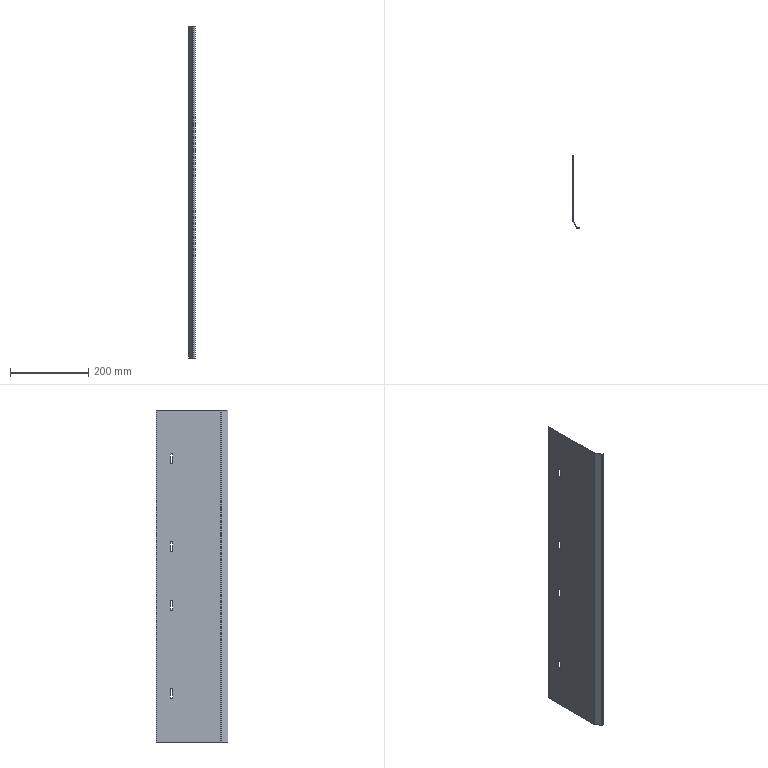Part | SolidWorks | features FlatPattern 1, ICE 1, SMBaseFlange 1, SheetMetal 1 | 1 solid | 42 faces | box 17 x 184.321 x 850 mm | volume 163173 mm3 | plane 26 | cylinder 16 | commonest cylinder face diameters 6 x12 2 x2 4 x2
STEP:
#1=CARTESIAN_POINT('',(0.,-37.,-290.));
#2=VERTEX_POINT('',#1);
#3=CARTESIAN_POINT('',(0.,-40.,-287.));
#4=VERTEX_POINT('',#3);
#5=CARTESIAN_POINT('',(0.,-40.,-290.));
#6=DIRECTION('',(1.,0.,0.));
#7=DIRECTION('',(0.,1.,0.));
#8=AXIS2_PLACEMENT_3D('',#5,#6,#7);
#9=CIRCLE('',#8,3.);
#10=EDGE_CURVE('',#2,#4,#9,.T.);
#11=ORIENTED_EDGE('',*,*,#10,.T.);
#12=CARTESIAN_POINT('',(-1.,-40.,-287.));
#13=VERTEX_POINT('',#12);
#14=CARTESIAN_POINT('',(9.,-40.,-287.));
#15=DIRECTION('',(-1.,0.,0.));
#16=VECTOR('',#15,1000.);
#17=LINE('',#14,#16);
#18=EDGE_CURVE('',#4,#13,#17,.T.);
#19=ORIENTED_EDGE('',*,*,#18,.T.);
#20=CARTESIAN_POINT('',(-1.,-37.,-290.));
#21=VERTEX_POINT('',#20);
#22=CARTESIAN_POINT('',(-1.,-40.,-290.));
#23=DIRECTION('',(-1.,0.,0.));
#24=DIRECTION('',(0.,0.,1.));
#25=AXIS2_PLACEMENT_3D('',#22,#23,#24);
#26=CIRCLE('',#25,3.);
#27=EDGE_CURVE('',#13,#21,#26,.T.);
#28=ORIENTED_EDGE('',*,*,#27,.T.);
#29=CARTESIAN_POINT('',(9.,-37.,-290.));
#30=DIRECTION('',(-1.,0.,0.));
#31=VECTOR('',#30,1000.);
#32=LINE('',#29,#31);
#33=EDGE_CURVE('',#2,#21,#32,.T.);
#34=ORIENTED_EDGE('',*,*,#33,.F.);
#35=EDGE_LOOP('',(#11,#19,#28,#34));
#36=FACE_OUTER_BOUND('',#35,.T.);
#37=CARTESIAN_POINT('',(9.,-40.,-290.));
#38=DIRECTION('',(-1.,0.,0.));
#39=DIRECTION('',(0.,0.,1.));
#40=AXIS2_PLACEMENT_3D('',#37,#38,#39);
#41=CYLINDRICAL_SURFACE('',#40,3.);
#42=ADVANCED_FACE('',(#36),#41,.F.);
#43=CARTESIAN_POINT('',(0.,-37.,85.));
#44=VERTEX_POINT('',#43);
#45=CARTESIAN_POINT('',(0.,-40.,88.));
#46=VERTEX_POINT('',#45);
#47=CARTESIAN_POINT('',(0.,-40.,85.));
#48=DIRECTION('',(1.,0.,0.));
#49=DIRECTION('',(0.,1.,0.));
#50=AXIS2_PLACEMENT_3D('',#47,#48,#49);
#51=CIRCLE('',#50,3.);
#52=EDGE_CURVE('',#44,#46,#51,.T.);
#53=ORIENTED_EDGE('',*,*,#52,.T.);
#54=CARTESIAN_POINT('',(-1.,-40.,88.));
#55=VERTEX_POINT('',#54);
#56=CARTESIAN_POINT('',(9.,-40.,88.));
#57=DIRECTION('',(-1.,0.,0.));
#58=VECTOR('',#57,1000.);
#59=LINE('',#56,#58);
#60=EDGE_CURVE('',#46,#55,#59,.T.);
#61=ORIENTED_EDGE('',*,*,#60,.T.);
#62=CARTESIAN_POINT('',(-1.,-37.,85.));
#63=VERTEX_POINT('',#62);
#64=CARTESIAN_POINT('',(-1.,-40.,85.));
#65=DIRECTION('',(-1.,0.,0.));
#66=DIRECTION('',(0.,0.,1.));
#67=AXIS2_PLACEMENT_3D('',#64,#65,#66);
#68=CIRCLE('',#67,3.);
#69=EDGE_CURVE('',#55,#63,#68,.T.);
#70=ORIENTED_EDGE('',*,*,#69,.T.);
#71=CARTESIAN_POINT('',(9.,-37.,85.));
#72=DIRECTION('',(-1.,0.,0.));
#73=VECTOR('',#72,1000.);
#74=LINE('',#71,#73);
#75=EDGE_CURVE('',#44,#63,#74,.T.);
#76=ORIENTED_EDGE('',*,*,#75,.F.);
#77=EDGE_LOOP('',(#53,#61,#70,#76));
#78=FACE_OUTER_BOUND('',#77,.T.);
#79=CARTESIAN_POINT('',(9.,-40.,85.));
#80=DIRECTION('',(-1.,0.,0.));
#81=DIRECTION('',(0.,0.,1.));
#82=AXIS2_PLACEMENT_3D('',#79,#80,#81);
#83=CYLINDRICAL_SURFACE('',#82,3.);
#84=ADVANCED_FACE('',(#78),#83,.F.);
#85=CARTESIAN_POINT('',(0.,-37.,310.));
#86=VERTEX_POINT('',#85);
#87=CARTESIAN_POINT('',(0.,-40.,313.));
#88=VERTEX_POINT('',#87);
#89=CARTESIAN_POINT('',(0.,-40.,310.));
#90=DIRECTION('',(1.,0.,0.));
#91=DIRECTION('',(0.,1.,0.));
#92=AXIS2_PLACEMENT_3D('',#89,#90,#91);
#93=CIRCLE('',#92,3.);
#94=EDGE_CURVE('',#86,#88,#93,.T.);
#95=ORIENTED_EDGE('',*,*,#94,.T.);
#96=CARTESIAN_POINT('',(-1.,-40.,313.));
#97=VERTEX_POINT('',#96);
#98=CARTESIAN_POINT('',(9.,-40.,313.));
#99=DIRECTION('',(-1.,0.,0.));
#100=VECTOR('',#99,1000.);
#101=LINE('',#98,#100);
#102=EDGE_CURVE('',#88,#97,#101,.T.);
#103=ORIENTED_EDGE('',*,*,#102,.T.);
#104=CARTESIAN_POINT('',(-1.,-37.,310.));
#105=VERTEX_POINT('',#104);
#106=CARTESIAN_POINT('',(-1.,-40.,310.));
#107=DIRECTION('',(-1.,0.,0.));
#108=DIRECTION('',(0.,0.,-1.));
#109=AXIS2_PLACEMENT_3D('',#106,#107,#108);
#110=CIRCLE('',#109,3.);
#111=EDGE_CURVE('',#97,#105,#110,.T.);
#112=ORIENTED_EDGE('',*,*,#111,.T.);
#113=CARTESIAN_POINT('',(9.,-37.,310.));
#114=DIRECTION('',(-1.,0.,0.));
#115=VECTOR('',#114,1000.);
#116=LINE('',#113,#115);
#117=EDGE_CURVE('',#86,#105,#116,.T.);
#118=ORIENTED_EDGE('',*,*,#117,.F.);
#119=EDGE_LOOP('',(#95,#103,#112,#118));
#120=FACE_OUTER_BOUND('',#119,.T.);
#121=CARTESIAN_POINT('',(9.,-40.,310.));
#122=DIRECTION('',(-1.,0.,0.));
#123=DIRECTION('',(0.,0.,1.));
#124=AXIS2_PLACEMENT_3D('',#121,#122,#123);
#125=CYLINDRICAL_SURFACE('',#124,3.);
#126=ADVANCED_FACE('',(#120),#125,.F.);
#127=CARTESIAN_POINT('',(0.,-37.,-65.));
#128=VERTEX_POINT('',#127);
#129=CARTESIAN_POINT('',(0.,-40.,-62.));
#130=VERTEX_POINT('',#129);
#131=CARTESIAN_POINT('',(0.,-40.,-65.));
#132=DIRECTION('',(1.,0.,0.));
#133=DIRECTION('',(0.,1.,0.));
#134=AXIS2_PLACEMENT_3D('',#131,#132,#133);
#135=CIRCLE('',#134,3.);
#136=EDGE_CURVE('',#128,#130,#135,.T.);
#137=ORIENTED_EDGE('',*,*,#136,.T.);
#138=CARTESIAN_POINT('',(-1.,-40.,-62.));
#139=VERTEX_POINT('',#138);
#140=CARTESIAN_POINT('',(9.,-40.,-62.));
#141=DIRECTION('',(-1.,0.,0.));
#142=VECTOR('',#141,1000.);
#143=LINE('',#140,#142);
#144=EDGE_CURVE('',#130,#139,#143,.T.);
#145=ORIENTED_EDGE('',*,*,#144,.T.);
#146=CARTESIAN_POINT('',(-1.,-37.,-65.));
#147=VERTEX_POINT('',#146);
#148=CARTESIAN_POINT('',(-1.,-40.,-65.));
#149=DIRECTION('',(-1.,0.,0.));
#150=DIRECTION('',(0.,0.,1.));
#151=AXIS2_PLACEMENT_3D('',#148,#149,#150);
#152=CIRCLE('',#151,3.);
#153=EDGE_CURVE('',#139,#147,#152,.T.);
#154=ORIENTED_EDGE('',*,*,#153,.T.);
#155=CARTESIAN_POINT('',(9.,-37.,-65.));
#156=DIRECTION('',(-1.,0.,0.));
#157=VECTOR('',#156,1000.);
#158=LINE('',#155,#157);
#159=EDGE_CURVE('',#128,#147,#158,.T.);
#160=ORIENTED_EDGE('',*,*,#159,.F.);
#161=EDGE_LOOP('',(#137,#145,#154,#160));
#162=FACE_OUTER_BOUND('',#161,.T.);
#163=CARTESIAN_POINT('',(9.,-40.,-65.));
#164=DIRECTION('',(-1.,0.,0.));
#165=DIRECTION('',(0.,0.,1.));
#166=AXIS2_PLACEMENT_3D('',#163,#164,#165);
#167=CYLINDRICAL_SURFACE('',#166,3.);
#168=ADVANCED_FACE('',(#162),#167,.F.);
#169=CARTESIAN_POINT('',(0.134,-166.232,425.));
#170=VERTEX_POINT('',#169);
#171=CARTESIAN_POINT('',(-0.7321,-166.732,425.));
#172=VERTEX_POINT('',#171);
#173=CARTESIAN_POINT('',(0.134,-166.232,425.));
#174=DIRECTION('',(-0.866,-0.5,0.));
#175=VECTOR('',#174,1000.);
#176=LINE('',#173,#175);
#177=EDGE_CURVE('',#170,#172,#176,.T.);
#178=ORIENTED_EDGE('',*,*,#177,.F.);
#179=CARTESIAN_POINT('',(0.,-165.732,425.));
#180=VERTEX_POINT('',#179);
#181=CARTESIAN_POINT('',(1.,-165.732,425.));
#182=DIRECTION('',(0.,0.,1.));
#183=DIRECTION('',(-1.,0.,0.));
#184=AXIS2_PLACEMENT_3D('',#181,#182,#183);
#185=CIRCLE('',#184,1.);
#186=EDGE_CURVE('',#180,#170,#185,.T.);
#187=ORIENTED_EDGE('',*,*,#186,.F.);
#188=CARTESIAN_POINT('',(-1.,-165.732,425.));
#189=VERTEX_POINT('',#188);
#190=CARTESIAN_POINT('',(-1.,-165.732,425.));
#191=DIRECTION('',(1.,0.,0.));
#192=VECTOR('',#191,1000.);
#193=LINE('',#190,#192);
#194=EDGE_CURVE('',#189,#180,#193,.T.);
#195=ORIENTED_EDGE('',*,*,#194,.F.);
#196=CARTESIAN_POINT('',(1.,-165.732,425.));
#197=DIRECTION('',(0.,0.,1.));
#198=DIRECTION('',(1.,0.,0.));
#199=AXIS2_PLACEMENT_3D('',#196,#197,#198);
#200=CIRCLE('',#199,2.);
#201=EDGE_CURVE('',#189,#172,#200,.T.);
#202=ORIENTED_EDGE('',*,*,#201,.T.);
#203=EDGE_LOOP('',(#178,#187,#195,#202));
#204=FACE_OUTER_BOUND('',#203,.T.);
#205=CARTESIAN_POINT('',(0.134,-166.232,425.));
#206=DIRECTION('',(0.,0.,1.));
#207=DIRECTION('',(1.,0.,0.));
#208=AXIS2_PLACEMENT_3D('',#205,#206,#207);
#209=PLANE('',#208);
#210=ADVANCED_FACE('',(#204),#209,.T.);
#211=CARTESIAN_POINT('',(9.711,-182.821,425.));
#212=VERTEX_POINT('',#211);
#213=CARTESIAN_POINT('',(0.,-166.,425.));
#214=DIRECTION('',(0.5,-0.866,0.));
#215=VECTOR('',#214,1000.);
#216=LINE('',#213,#215);
#217=EDGE_CURVE('',#170,#212,#216,.T.);
#218=ORIENTED_EDGE('',*,*,#217,.F.);
#219=ORIENTED_EDGE('',*,*,#177,.T.);
#220=CARTESIAN_POINT('',(8.845,-183.321,425.));
#221=VERTEX_POINT('',#220);
#222=CARTESIAN_POINT('',(-0.866,-166.5,425.));
#223=DIRECTION('',(0.5,-0.866,0.));
#224=VECTOR('',#223,1000.);
#225=LINE('',#222,#224);
#226=EDGE_CURVE('',#172,#221,#225,.T.);
#227=ORIENTED_EDGE('',*,*,#226,.T.);
#228=CARTESIAN_POINT('',(8.845,-183.321,425.));
#229=DIRECTION('',(0.866,0.5,0.));
#230=VECTOR('',#229,1000.);
#231=LINE('',#228,#230);
#232=EDGE_CURVE('',#221,#212,#231,.T.);
#233=ORIENTED_EDGE('',*,*,#232,.T.);
#234=EDGE_LOOP('',(#218,#219,#227,#233));
#235=FACE_OUTER_BOUND('',#234,.T.);
#236=CARTESIAN_POINT('',(-1.,-165.732,425.));
#237=DIRECTION('',(0.,0.,1.));
#238=DIRECTION('',(1.,0.,0.));
#239=AXIS2_PLACEMENT_3D('',#236,#237,#238);
#240=PLANE('',#239);
#241=ADVANCED_FACE('',(#235),#240,.T.);
#242=CARTESIAN_POINT('',(0.,-165.732,-425.));
#243=VERTEX_POINT('',#242);
#244=CARTESIAN_POINT('',(-1.,-165.732,-425.));
#245=VERTEX_POINT('',#244);
#246=CARTESIAN_POINT('',(0.,-165.732,-425.));
#247=DIRECTION('',(-1.,0.,0.));
#248=VECTOR('',#247,1000.);
#249=LINE('',#246,#248);
#250=EDGE_CURVE('',#243,#245,#249,.T.);
#251=ORIENTED_EDGE('',*,*,#250,.F.);
#252=CARTESIAN_POINT('',(0.134,-166.232,-425.));
#253=VERTEX_POINT('',#252);
#254=CARTESIAN_POINT('',(1.,-165.732,-425.));
#255=DIRECTION('',(0.,0.,1.));
#256=DIRECTION('',(-1.,0.,0.));
#257=AXIS2_PLACEMENT_3D('',#254,#255,#256);
#258=CIRCLE('',#257,1.);
#259=EDGE_CURVE('',#243,#253,#258,.T.);
#260=ORIENTED_EDGE('',*,*,#259,.T.);
#261=CARTESIAN_POINT('',(-0.7321,-166.732,-425.));
#262=VERTEX_POINT('',#261);
#263=CARTESIAN_POINT('',(-0.7321,-166.732,-425.));
#264=DIRECTION('',(0.866,0.5,0.));
#265=VECTOR('',#264,1000.);
#266=LINE('',#263,#265);
#267=EDGE_CURVE('',#262,#253,#266,.T.);
#268=ORIENTED_EDGE('',*,*,#267,.F.);
#269=CARTESIAN_POINT('',(1.,-165.732,-425.));
#270=DIRECTION('',(0.,0.,1.));
#271=DIRECTION('',(1.,0.,0.));
#272=AXIS2_PLACEMENT_3D('',#269,#270,#271);
#273=CIRCLE('',#272,2.);
#274=EDGE_CURVE('',#245,#262,#273,.T.);
#275=ORIENTED_EDGE('',*,*,#274,.F.);
#276=EDGE_LOOP('',(#251,#260,#268,#275));
#277=FACE_OUTER_BOUND('',#276,.T.);
#278=CARTESIAN_POINT('',(0.,-165.732,-425.));
#279=DIRECTION('',(0.,0.,-1.));
#280=DIRECTION('',(-1.,0.,0.));
#281=AXIS2_PLACEMENT_3D('',#278,#279,#280);
#282=PLANE('',#281);
#283=ADVANCED_FACE('',(#277),#282,.T.);
#284=CARTESIAN_POINT('',(0.,0.,-425.));
#285=VERTEX_POINT('',#284);
#286=CARTESIAN_POINT('',(0.,0.,-425.));
#287=DIRECTION('',(0.,-1.,0.));
#288=VECTOR('',#287,1000.);
#289=LINE('',#286,#288);
#290=EDGE_CURVE('',#285,#243,#289,.T.);
#291=ORIENTED_EDGE('',*,*,#290,.T.);
#292=ORIENTED_EDGE('',*,*,#250,.T.);
#293=CARTESIAN_POINT('',(-1.,0.,-425.));
#294=VERTEX_POINT('',#293);
#295=CARTESIAN_POINT('',(-1.,0.,-425.));
#296=DIRECTION('',(0.,-1.,0.));
#297=VECTOR('',#296,1000.);
#298=LINE('',#295,#297);
#299=EDGE_CURVE('',#294,#245,#298,.T.);
#300=ORIENTED_EDGE('',*,*,#299,.F.);
#301=CARTESIAN_POINT('',(-1.,0.,-425.));
#302=DIRECTION('',(1.,0.,0.));
#303=VECTOR('',#302,1000.);
#304=LINE('',#301,#303);
#305=EDGE_CURVE('',#294,#285,#304,.T.);
#306=ORIENTED_EDGE('',*,*,#305,.T.);
#307=EDGE_LOOP('',(#291,#292,#300,#306));
#308=FACE_OUTER_BOUND('',#307,.T.);
#309=CARTESIAN_POINT('',(-0.7321,-166.732,-425.));
#310=DIRECTION('',(0.,0.,-1.));
#311=DIRECTION('',(-1.,0.,0.));
#312=AXIS2_PLACEMENT_3D('',#309,#310,#311);
#313=PLANE('',#312);
#314=ADVANCED_FACE('',(#308),#313,.T.);
#315=CARTESIAN_POINT('',(10.577,-183.321,425.));
#316=VERTEX_POINT('',#315);
#317=CARTESIAN_POINT('',(10.577,-184.321,425.));
#318=VERTEX_POINT('',#317);
#319=CARTESIAN_POINT('',(10.577,-183.321,425.));
#320=DIRECTION('',(0.,-1.,0.));
#321=VECTOR('',#320,1000.);
#322=LINE('',#319,#321);
#323=EDGE_CURVE('',#316,#318,#322,.T.);
#324=ORIENTED_EDGE('',*,*,#323,.F.);
#325=CARTESIAN_POINT('',(10.577,-182.321,425.));
#326=DIRECTION('',(0.,0.,1.));
#327=DIRECTION('',(-1.,0.,0.));
#328=AXIS2_PLACEMENT_3D('',#325,#326,#327);
#329=CIRCLE('',#328,1.);
#330=EDGE_CURVE('',#212,#316,#329,.T.);
#331=ORIENTED_EDGE('',*,*,#330,.F.);
#332=ORIENTED_EDGE('',*,*,#232,.F.);
#333=CARTESIAN_POINT('',(10.577,-182.321,425.));
#334=DIRECTION('',(0.,0.,1.));
#335=DIRECTION('',(1.,0.,0.));
#336=AXIS2_PLACEMENT_3D('',#333,#334,#335);
#337=CIRCLE('',#336,2.);
#338=EDGE_CURVE('',#221,#318,#337,.T.);
#339=ORIENTED_EDGE('',*,*,#338,.T.);
#340=EDGE_LOOP('',(#324,#331,#332,#339));
#341=FACE_OUTER_BOUND('',#340,.T.);
#342=CARTESIAN_POINT('',(10.577,-183.321,425.));
#343=DIRECTION('',(0.,0.,1.));
#344=DIRECTION('',(1.,0.,0.));
#345=AXIS2_PLACEMENT_3D('',#342,#343,#344);
#346=PLANE('',#345);
#347=ADVANCED_FACE('',(#341),#346,.T.);
#348=CARTESIAN_POINT('',(16.,-183.321,425.));
#349=VERTEX_POINT('',#348);
#350=CARTESIAN_POINT('',(10.,-183.321,425.));
#351=DIRECTION('',(1.,0.,0.));
#352=VECTOR('',#351,1000.);
#353=LINE('',#350,#352);
#354=EDGE_CURVE('',#316,#349,#353,.T.);
#355=ORIENTED_EDGE('',*,*,#354,.F.);
#356=ORIENTED_EDGE('',*,*,#323,.T.);
#357=CARTESIAN_POINT('',(16.,-184.321,425.));
#358=VERTEX_POINT('',#357);
#359=CARTESIAN_POINT('',(10.,-184.321,425.));
#360=DIRECTION('',(1.,0.,0.));
#361=VECTOR('',#360,1000.);
#362=LINE('',#359,#361);
#363=EDGE_CURVE('',#318,#358,#362,.T.);
#364=ORIENTED_EDGE('',*,*,#363,.T.);
#365=CARTESIAN_POINT('',(16.,-183.321,425.));
#366=DIRECTION('',(0.,-1.,0.));
#367=VECTOR('',#366,1000.);
#368=LINE('',#365,#367);
#369=EDGE_CURVE('',#349,#358,#368,.T.);
#370=ORIENTED_EDGE('',*,*,#369,.F.);
#371=EDGE_LOOP('',(#355,#356,#364,#370));
#372=FACE_OUTER_BOUND('',#371,.T.);
#373=CARTESIAN_POINT('',(8.845,-183.321,425.));
#374=DIRECTION('',(0.,0.,1.));
#375=DIRECTION('',(1.,0.,0.));
#376=AXIS2_PLACEMENT_3D('',#373,#374,#375);
#377=PLANE('',#376);
#378=ADVANCED_FACE('',(#372),#377,.T.);
#379=CARTESIAN_POINT('',(9.711,-182.821,-425.));
#380=VERTEX_POINT('',#379);
#381=CARTESIAN_POINT('',(8.845,-183.321,-425.));
#382=VERTEX_POINT('',#381);
#383=CARTESIAN_POINT('',(9.711,-182.821,-425.));
#384=DIRECTION('',(-0.866,-0.5,0.));
#385=VECTOR('',#384,1000.);
#386=LINE('',#383,#385);
#387=EDGE_CURVE('',#380,#382,#386,.T.);
#388=ORIENTED_EDGE('',*,*,#387,.F.);
#389=CARTESIAN_POINT('',(10.577,-183.321,-425.));
#390=VERTEX_POINT('',#389);
#391=CARTESIAN_POINT('',(10.577,-182.321,-425.));
#392=DIRECTION('',(0.,0.,1.));
#393=DIRECTION('',(-1.,0.,0.));
#394=AXIS2_PLACEMENT_3D('',#391,#392,#393);
#395=CIRCLE('',#394,1.);
#396=EDGE_CURVE('',#380,#390,#395,.T.);
#397=ORIENTED_EDGE('',*,*,#396,.T.);
#398=CARTESIAN_POINT('',(10.577,-184.321,-425.));
#399=VERTEX_POINT('',#398);
#400=CARTESIAN_POINT('',(10.577,-184.321,-425.));
#401=DIRECTION('',(0.,1.,0.));
#402=VECTOR('',#401,1000.);
#403=LINE('',#400,#402);
#404=EDGE_CURVE('',#399,#390,#403,.T.);
#405=ORIENTED_EDGE('',*,*,#404,.F.);
#406=CARTESIAN_POINT('',(10.577,-182.321,-425.));
#407=DIRECTION('',(0.,0.,1.));
#408=DIRECTION('',(1.,0.,0.));
#409=AXIS2_PLACEMENT_3D('',#406,#407,#408);
#410=CIRCLE('',#409,2.);
#411=EDGE_CURVE('',#382,#399,#410,.T.);
#412=ORIENTED_EDGE('',*,*,#411,.F.);
#413=EDGE_LOOP('',(#388,#397,#405,#412));
#414=FACE_OUTER_BOUND('',#413,.T.);
#415=CARTESIAN_POINT('',(9.711,-182.821,-425.));
#416=DIRECTION('',(0.,0.,-1.));
#417=DIRECTION('',(-1.,0.,0.));
#418=AXIS2_PLACEMENT_3D('',#415,#416,#417);
#419=PLANE('',#418);
#420=ADVANCED_FACE('',(#414),#419,.T.);
#421=CARTESIAN_POINT('',(0.,-166.,-425.));
#422=DIRECTION('',(0.5,-0.866,0.));
#423=VECTOR('',#422,1000.);
#424=LINE('',#421,#423);
#425=EDGE_CURVE('',#253,#380,#424,.T.);
#426=ORIENTED_EDGE('',*,*,#425,.T.);
#427=ORIENTED_EDGE('',*,*,#387,.T.);
#428=CARTESIAN_POINT('',(-0.866,-166.5,-425.));
#429=DIRECTION('',(0.5,-0.866,0.));
#430=VECTOR('',#429,1000.);
#431=LINE('',#428,#430);
#432=EDGE_CURVE('',#262,#382,#431,.T.);
#433=ORIENTED_EDGE('',*,*,#432,.F.);
#434=ORIENTED_EDGE('',*,*,#267,.T.);
#435=EDGE_LOOP('',(#426,#427,#433,#434));
#436=FACE_OUTER_BOUND('',#435,.T.);
#437=CARTESIAN_POINT('',(10.577,-184.321,-425.));
#438=DIRECTION('',(0.,0.,-1.));
#439=DIRECTION('',(-1.,0.,0.));
#440=AXIS2_PLACEMENT_3D('',#437,#438,#439);
#441=PLANE('',#440);
#442=ADVANCED_FACE('',(#436),#441,.T.);
#443=CARTESIAN_POINT('',(16.,-184.321,-425.));
#444=VERTEX_POINT('',#443);
#445=CARTESIAN_POINT('',(10.,-184.321,-425.));
#446=DIRECTION('',(1.,0.,0.));
#447=VECTOR('',#446,1000.);
#448=LINE('',#445,#447);
#449=EDGE_CURVE('',#399,#444,#448,.T.);
#450=ORIENTED_EDGE('',*,*,#449,.T.);
#451=CARTESIAN_POINT('',(16.,-184.321,425.));
#452=DIRECTION('',(0.,0.,-1.));
#453=VECTOR('',#452,1000.);
#454=LINE('',#451,#453);
#455=EDGE_CURVE('',#358,#444,#454,.T.);
#456=ORIENTED_EDGE('',*,*,#455,.F.);
#457=ORIENTED_EDGE('',*,*,#363,.F.);
#458=CARTESIAN_POINT('',(10.577,-184.321,425.));
#459=DIRECTION('',(0.,0.,-1.));
#460=VECTOR('',#459,1000.);
#461=LINE('',#458,#460);
#462=EDGE_CURVE('',#318,#399,#461,.T.);
#463=ORIENTED_EDGE('',*,*,#462,.T.);
#464=EDGE_LOOP('',(#450,#456,#457,#463));
#465=FACE_OUTER_BOUND('',#464,.T.);
#466=CARTESIAN_POINT('',(10.,-184.321,425.));
#467=DIRECTION('',(0.,1.,0.));
#468=DIRECTION('',(-1.,0.,0.));
#469=AXIS2_PLACEMENT_3D('',#466,#467,#468);
#470=PLANE('',#469);
#471=ADVANCED_FACE('',(#465),#470,.F.);
#472=CARTESIAN_POINT('',(16.,-183.321,-425.));
#473=VERTEX_POINT('',#472);
#474=CARTESIAN_POINT('',(16.,-183.321,-425.));
#475=DIRECTION('',(0.,-1.,0.));
#476=VECTOR('',#475,1000.);
#477=LINE('',#474,#476);
#478=EDGE_CURVE('',#473,#444,#477,.T.);
#479=ORIENTED_EDGE('',*,*,#478,.F.);
#480=CARTESIAN_POINT('',(16.,-183.321,425.));
#481=DIRECTION('',(0.,0.,-1.));
#482=VECTOR('',#481,1000.);
#483=LINE('',#480,#482);
#484=EDGE_CURVE('',#349,#473,#483,.T.);
#485=ORIENTED_EDGE('',*,*,#484,.F.);
#486=ORIENTED_EDGE('',*,*,#369,.T.);
#487=ORIENTED_EDGE('',*,*,#455,.T.);
#488=EDGE_LOOP('',(#479,#485,#486,#487));
#489=FACE_OUTER_BOUND('',#488,.T.);
#490=CARTESIAN_POINT('',(16.,-183.321,425.));
#491=DIRECTION('',(1.,0.,0.));
#492=DIRECTION('',(0.,1.,0.));
#493=AXIS2_PLACEMENT_3D('',#490,#491,#492);
#494=PLANE('',#493);
#495=ADVANCED_FACE('',(#489),#494,.T.);
#496=CARTESIAN_POINT('',(10.,-183.321,-425.));
#497=DIRECTION('',(1.,0.,0.));
#498=VECTOR('',#497,1000.);
#499=LINE('',#496,#498);
#500=EDGE_CURVE('',#390,#473,#499,.T.);
#501=ORIENTED_EDGE('',*,*,#500,.F.);
#502=CARTESIAN_POINT('',(10.577,-183.321,425.));
#503=DIRECTION('',(0.,0.,-1.));
#504=VECTOR('',#503,1000.);
#505=LINE('',#502,#504);
#506=EDGE_CURVE('',#316,#390,#505,.T.);
#507=ORIENTED_EDGE('',*,*,#506,.F.);
#508=ORIENTED_EDGE('',*,*,#354,.T.);
#509=ORIENTED_EDGE('',*,*,#484,.T.);
#510=EDGE_LOOP('',(#501,#507,#508,#509));
#511=FACE_OUTER_BOUND('',#510,.T.);
#512=CARTESIAN_POINT('',(10.,-183.321,425.));
#513=DIRECTION('',(0.,1.,0.));
#514=DIRECTION('',(-1.,0.,0.));
#515=AXIS2_PLACEMENT_3D('',#512,#513,#514);
#516=PLANE('',#515);
#517=ADVANCED_FACE('',(#511),#516,.T.);
#518=ORIENTED_EDGE('',*,*,#396,.F.);
#519=CARTESIAN_POINT('',(9.711,-182.821,425.));
#520=DIRECTION('',(0.,0.,-1.));
#521=VECTOR('',#520,1000.);
#522=LINE('',#519,#521);
#523=EDGE_CURVE('',#212,#380,#522,.T.);
#524=ORIENTED_EDGE('',*,*,#523,.F.);
#525=ORIENTED_EDGE('',*,*,#330,.T.);
#526=ORIENTED_EDGE('',*,*,#506,.T.);
#527=EDGE_LOOP('',(#518,#524,#525,#526));
#528=FACE_OUTER_BOUND('',#527,.T.);
#529=CARTESIAN_POINT('',(10.577,-182.321,425.));
#530=DIRECTION('',(0.,0.,-1.));
#531=DIRECTION('',(-1.,0.,0.));
#532=AXIS2_PLACEMENT_3D('',#529,#530,#531);
#533=CYLINDRICAL_SURFACE('',#532,1.);
#534=ADVANCED_FACE('',(#528),#533,.F.);
#535=ORIENTED_EDGE('',*,*,#425,.F.);
#536=CARTESIAN_POINT('',(0.134,-166.232,425.));
#537=DIRECTION('',(0.,0.,-1.));
#538=VECTOR('',#537,1000.);
#539=LINE('',#536,#538);
#540=EDGE_CURVE('',#170,#253,#539,.T.);
#541=ORIENTED_EDGE('',*,*,#540,.F.);
#542=ORIENTED_EDGE('',*,*,#217,.T.);
#543=ORIENTED_EDGE('',*,*,#523,.T.);
#544=EDGE_LOOP('',(#535,#541,#542,#543));
#545=FACE_OUTER_BOUND('',#544,.T.);
#546=CARTESIAN_POINT('',(0.,-166.,425.));
#547=DIRECTION('',(0.866,0.5,0.));
#548=DIRECTION('',(-0.5,0.866,0.));
#549=AXIS2_PLACEMENT_3D('',#546,#547,#548);
#550=PLANE('',#549);
#551=ADVANCED_FACE('',(#545),#550,.T.);
#552=ORIENTED_EDGE('',*,*,#259,.F.);
#553=CARTESIAN_POINT('',(0.,-165.732,425.));
#554=DIRECTION('',(0.,0.,-1.));
#555=VECTOR('',#554,1000.);
#556=LINE('',#553,#555);
#557=EDGE_CURVE('',#180,#243,#556,.T.);
#558=ORIENTED_EDGE('',*,*,#557,.F.);
#559=ORIENTED_EDGE('',*,*,#186,.T.);
#560=ORIENTED_EDGE('',*,*,#540,.T.);
#561=EDGE_LOOP('',(#552,#558,#559,#560));
#562=FACE_OUTER_BOUND('',#561,.T.);
#563=CARTESIAN_POINT('',(1.,-165.732,425.));
#564=DIRECTION('',(0.,0.,-1.));
#565=DIRECTION('',(-1.,0.,0.));
#566=AXIS2_PLACEMENT_3D('',#563,#564,#565);
#567=CYLINDRICAL_SURFACE('',#566,1.);
#568=ADVANCED_FACE('',(#562),#567,.F.);
#569=CARTESIAN_POINT('',(0.,-43.,-310.));
#570=VERTEX_POINT('',#569);
#571=CARTESIAN_POINT('',(0.,-37.,-310.));
#572=VERTEX_POINT('',#571);
#573=CARTESIAN_POINT('',(0.,-40.,-310.));
#574=DIRECTION('',(1.,0.,0.));
#575=DIRECTION('',(0.,1.,0.));
#576=AXIS2_PLACEMENT_3D('',#573,#574,#575);
#577=CIRCLE('',#576,3.);
#578=EDGE_CURVE('',#570,#572,#577,.T.);
#579=ORIENTED_EDGE('',*,*,#578,.F.);
#580=CARTESIAN_POINT('',(0.,-43.,-290.));
#581=VERTEX_POINT('',#580);
#582=CARTESIAN_POINT('',(0.,-43.,425.));
#583=DIRECTION('',(0.,0.,-1.));
#584=VECTOR('',#583,1000.);
#585=LINE('',#582,#584);
#586=EDGE_CURVE('',#581,#570,#585,.T.);
#587=ORIENTED_EDGE('',*,*,#586,.F.);
#588=CARTESIAN_POINT('',(0.,-40.,-290.));
#589=DIRECTION('',(1.,0.,0.));
#590=DIRECTION('',(0.,1.,0.));
#591=AXIS2_PLACEMENT_3D('',#588,#589,#590);
#592=CIRCLE('',#591,3.);
#593=EDGE_CURVE('',#4,#581,#592,.T.);
#594=ORIENTED_EDGE('',*,*,#593,.F.);
#595=ORIENTED_EDGE('',*,*,#10,.F.);
#596=CARTESIAN_POINT('',(0.,-37.,425.));
#597=DIRECTION('',(0.,0.,1.));
#598=VECTOR('',#597,1000.);
#599=LINE('',#596,#598);
#600=EDGE_CURVE('',#572,#2,#599,.T.);
#601=ORIENTED_EDGE('',*,*,#600,.F.);
#602=EDGE_LOOP('',(#579,#587,#594,#595,#601));
#603=FACE_BOUND('',#602,.T.);
#604=CARTESIAN_POINT('',(0.,-43.,65.));
#605=VERTEX_POINT('',#604);
#606=CARTESIAN_POINT('',(0.,-37.,65.));
#607=VERTEX_POINT('',#606);
#608=CARTESIAN_POINT('',(0.,-40.,65.));
#609=DIRECTION('',(1.,0.,0.));
#610=DIRECTION('',(0.,1.,0.));
#611=AXIS2_PLACEMENT_3D('',#608,#609,#610);
#612=CIRCLE('',#611,3.);
#613=EDGE_CURVE('',#605,#607,#612,.T.);
#614=ORIENTED_EDGE('',*,*,#613,.F.);
#615=CARTESIAN_POINT('',(0.,-43.,85.));
#616=VERTEX_POINT('',#615);
#617=CARTESIAN_POINT('',(0.,-43.,425.));
#618=DIRECTION('',(0.,0.,-1.));
#619=VECTOR('',#618,1000.);
#620=LINE('',#617,#619);
#621=EDGE_CURVE('',#616,#605,#620,.T.);
#622=ORIENTED_EDGE('',*,*,#621,.F.);
#623=CARTESIAN_POINT('',(0.,-40.,85.));
#624=DIRECTION('',(1.,0.,0.));
#625=DIRECTION('',(0.,1.,0.));
#626=AXIS2_PLACEMENT_3D('',#623,#624,#625);
#627=CIRCLE('',#626,3.);
#628=EDGE_CURVE('',#46,#616,#627,.T.);
#629=ORIENTED_EDGE('',*,*,#628,.F.);
#630=ORIENTED_EDGE('',*,*,#52,.F.);
#631=CARTESIAN_POINT('',(0.,-37.,425.));
#632=DIRECTION('',(0.,0.,1.));
#633=VECTOR('',#632,1000.);
#634=LINE('',#631,#633);
#635=EDGE_CURVE('',#607,#44,#634,.T.);
#636=ORIENTED_EDGE('',*,*,#635,.F.);
#637=EDGE_LOOP('',(#614,#622,#629,#630,#636));
#638=FACE_BOUND('',#637,.T.);
#639=ORIENTED_EDGE('',*,*,#94,.F.);
#640=CARTESIAN_POINT('',(0.,-37.,290.));
#641=VERTEX_POINT('',#640);
#642=CARTESIAN_POINT('',(0.,-37.,425.));
#643=DIRECTION('',(0.,0.,1.));
#644=VECTOR('',#643,1000.);
#645=LINE('',#642,#644);
#646=EDGE_CURVE('',#641,#86,#645,.T.);
#647=ORIENTED_EDGE('',*,*,#646,.F.);
#648=CARTESIAN_POINT('',(0.,-43.,290.));
#649=VERTEX_POINT('',#648);
#650=CARTESIAN_POINT('',(0.,-40.,290.));
#651=DIRECTION('',(1.,0.,0.));
#652=DIRECTION('',(0.,1.,0.));
#653=AXIS2_PLACEMENT_3D('',#650,#651,#652);
#654=CIRCLE('',#653,3.);
#655=EDGE_CURVE('',#649,#641,#654,.T.);
#656=ORIENTED_EDGE('',*,*,#655,.F.);
#657=CARTESIAN_POINT('',(0.,-43.,310.));
#658=VERTEX_POINT('',#657);
#659=CARTESIAN_POINT('',(0.,-43.,425.));
#660=DIRECTION('',(0.,0.,-1.));
#661=VECTOR('',#660,1000.);
#662=LINE('',#659,#661);
#663=EDGE_CURVE('',#658,#649,#662,.T.);
#664=ORIENTED_EDGE('',*,*,#663,.F.);
#665=CARTESIAN_POINT('',(0.,-40.,310.));
#666=DIRECTION('',(1.,0.,0.));
#667=DIRECTION('',(0.,1.,0.));
#668=AXIS2_PLACEMENT_3D('',#665,#666,#667);
#669=CIRCLE('',#668,3.);
#670=EDGE_CURVE('',#88,#658,#669,.T.);
#671=ORIENTED_EDGE('',*,*,#670,.F.);
#672=EDGE_LOOP('',(#639,#647,#656,#664,#671));
#673=FACE_BOUND('',#672,.T.);
#674=CARTESIAN_POINT('',(0.,-43.,-85.));
#675=VERTEX_POINT('',#674);
#676=CARTESIAN_POINT('',(0.,-37.,-85.));
#677=VERTEX_POINT('',#676);
#678=CARTESIAN_POINT('',(0.,-40.,-85.));
#679=DIRECTION('',(1.,0.,0.));
#680=DIRECTION('',(0.,1.,0.));
#681=AXIS2_PLACEMENT_3D('',#678,#679,#680);
#682=CIRCLE('',#681,3.);
#683=EDGE_CURVE('',#675,#677,#682,.T.);
#684=ORIENTED_EDGE('',*,*,#683,.F.);
#685=CARTESIAN_POINT('',(0.,-43.,-65.));
#686=VERTEX_POINT('',#685);
#687=CARTESIAN_POINT('',(0.,-43.,425.));
#688=DIRECTION('',(0.,0.,-1.));
#689=VECTOR('',#688,1000.);
#690=LINE('',#687,#689);
#691=EDGE_CURVE('',#686,#675,#690,.T.);
#692=ORIENTED_EDGE('',*,*,#691,.F.);
#693=CARTESIAN_POINT('',(0.,-40.,-65.));
#694=DIRECTION('',(1.,0.,0.));
#695=DIRECTION('',(0.,1.,0.));
#696=AXIS2_PLACEMENT_3D('',#693,#694,#695);
#697=CIRCLE('',#696,3.);
#698=EDGE_CURVE('',#130,#686,#697,.T.);
#699=ORIENTED_EDGE('',*,*,#698,.F.);
#700=ORIENTED_EDGE('',*,*,#136,.F.);
#701=CARTESIAN_POINT('',(0.,-37.,425.));
#702=DIRECTION('',(0.,0.,1.));
#703=VECTOR('',#702,1000.);
#704=LINE('',#701,#703);
#705=EDGE_CURVE('',#677,#128,#704,.T.);
#706=ORIENTED_EDGE('',*,*,#705,.F.);
#707=EDGE_LOOP('',(#684,#692,#699,#700,#706));
#708=FACE_BOUND('',#707,.T.);
#709=ORIENTED_EDGE('',*,*,#290,.F.);
#710=CARTESIAN_POINT('',(0.,0.,425.));
#711=VERTEX_POINT('',#710);
#712=CARTESIAN_POINT('',(0.,0.,425.));
#713=DIRECTION('',(0.,0.,-1.));
#714=VECTOR('',#713,1000.);
#715=LINE('',#712,#714);
#716=EDGE_CURVE('',#711,#285,#715,.T.);
#717=ORIENTED_EDGE('',*,*,#716,.F.);
#718=CARTESIAN_POINT('',(0.,0.,425.));
#719=DIRECTION('',(0.,-1.,0.));
#720=VECTOR('',#719,1000.);
#721=LINE('',#718,#720);
#722=EDGE_CURVE('',#711,#180,#721,.T.);
#723=ORIENTED_EDGE('',*,*,#722,.T.);
#724=ORIENTED_EDGE('',*,*,#557,.T.);
#725=EDGE_LOOP('',(#709,#717,#723,#724));
#726=FACE_OUTER_BOUND('',#725,.T.);
#727=CARTESIAN_POINT('',(0.,0.,425.));
#728=DIRECTION('',(1.,0.,0.));
#729=DIRECTION('',(0.,1.,0.));
#730=AXIS2_PLACEMENT_3D('',#727,#728,#729);
#731=PLANE('',#730);
#732=ADVANCED_FACE('',(#603,#638,#673,#708,#726),#731,.T.);
#733=ORIENTED_EDGE('',*,*,#305,.F.);
#734=CARTESIAN_POINT('',(-1.,0.,425.));
#735=VERTEX_POINT('',#734);
#736=CARTESIAN_POINT('',(-1.,0.,425.));
#737=DIRECTION('',(0.,0.,-1.));
#738=VECTOR('',#737,1000.);
#739=LINE('',#736,#738);
#740=EDGE_CURVE('',#735,#294,#739,.T.);
#741=ORIENTED_EDGE('',*,*,#740,.F.);
#742=CARTESIAN_POINT('',(-1.,0.,425.));
#743=DIRECTION('',(1.,0.,0.));
#744=VECTOR('',#743,1000.);
#745=LINE('',#742,#744);
#746=EDGE_CURVE('',#735,#711,#745,.T.);
#747=ORIENTED_EDGE('',*,*,#746,.T.);
#748=ORIENTED_EDGE('',*,*,#716,.T.);
#749=EDGE_LOOP('',(#733,#741,#747,#748));
#750=FACE_OUTER_BOUND('',#749,.T.);
#751=CARTESIAN_POINT('',(-1.,0.,425.));
#752=DIRECTION('',(0.,1.,0.));
#753=DIRECTION('',(-1.,0.,0.));
#754=AXIS2_PLACEMENT_3D('',#751,#752,#753);
#755=PLANE('',#754);
#756=ADVANCED_FACE('',(#750),#755,.T.);
#757=CARTESIAN_POINT('',(-1.,-43.,-310.));
#758=VERTEX_POINT('',#757);
#759=CARTESIAN_POINT('',(-1.,-43.,-290.));
#760=VERTEX_POINT('',#759);
#761=CARTESIAN_POINT('',(-1.,-43.,-310.));
#762=DIRECTION('',(0.,0.,1.));
#763=VECTOR('',#762,1000.);
#764=LINE('',#761,#763);
#765=EDGE_CURVE('',#758,#760,#764,.T.);
#766=ORIENTED_EDGE('',*,*,#765,.F.);
#767=CARTESIAN_POINT('',(-1.,-37.,-310.));
#768=VERTEX_POINT('',#767);
#769=CARTESIAN_POINT('',(-1.,-40.,-310.));
#770=DIRECTION('',(-1.,0.,0.));
#771=DIRECTION('',(0.,0.,1.));
#772=AXIS2_PLACEMENT_3D('',#769,#770,#771);
#773=CIRCLE('',#772,3.);
#774=EDGE_CURVE('',#768,#758,#773,.T.);
#775=ORIENTED_EDGE('',*,*,#774,.F.);
#776=CARTESIAN_POINT('',(-1.,-37.,-310.));
#777=DIRECTION('',(0.,0.,-1.));
#778=VECTOR('',#777,1000.);
#779=LINE('',#776,#778);
#780=EDGE_CURVE('',#21,#768,#779,.T.);
#781=ORIENTED_EDGE('',*,*,#780,.F.);
#782=ORIENTED_EDGE('',*,*,#27,.F.);
#783=CARTESIAN_POINT('',(-1.,-40.,-290.));
#784=DIRECTION('',(-1.,0.,0.));
#785=DIRECTION('',(0.,0.,1.));
#786=AXIS2_PLACEMENT_3D('',#783,#784,#785);
#787=CIRCLE('',#786,3.);
#788=EDGE_CURVE('',#760,#13,#787,.T.);
#789=ORIENTED_EDGE('',*,*,#788,.F.);
#790=EDGE_LOOP('',(#766,#775,#781,#782,#789));
#791=FACE_BOUND('',#790,.T.);
#792=CARTESIAN_POINT('',(-1.,-43.,65.));
#793=VERTEX_POINT('',#792);
#794=CARTESIAN_POINT('',(-1.,-43.,85.));
#795=VERTEX_POINT('',#794);
#796=CARTESIAN_POINT('',(-1.,-43.,65.));
#797=DIRECTION('',(0.,0.,1.));
#798=VECTOR('',#797,1000.);
#799=LINE('',#796,#798);
#800=EDGE_CURVE('',#793,#795,#799,.T.);
#801=ORIENTED_EDGE('',*,*,#800,.F.);
#802=CARTESIAN_POINT('',(-1.,-37.,65.));
#803=VERTEX_POINT('',#802);
#804=CARTESIAN_POINT('',(-1.,-40.,65.));
#805=DIRECTION('',(-1.,0.,0.));
#806=DIRECTION('',(0.,0.,1.));
#807=AXIS2_PLACEMENT_3D('',#804,#805,#806);
#808=CIRCLE('',#807,3.);
#809=EDGE_CURVE('',#803,#793,#808,.T.);
#810=ORIENTED_EDGE('',*,*,#809,.F.);
#811=CARTESIAN_POINT('',(-1.,-37.,65.));
#812=DIRECTION('',(0.,0.,-1.));
#813=VECTOR('',#812,1000.);
#814=LINE('',#811,#813);
#815=EDGE_CURVE('',#63,#803,#814,.T.);
#816=ORIENTED_EDGE('',*,*,#815,.F.);
#817=ORIENTED_EDGE('',*,*,#69,.F.);
#818=CARTESIAN_POINT('',(-1.,-40.,85.));
#819=DIRECTION('',(-1.,0.,0.));
#820=DIRECTION('',(0.,0.,1.));
#821=AXIS2_PLACEMENT_3D('',#818,#819,#820);
#822=CIRCLE('',#821,3.);
#823=EDGE_CURVE('',#795,#55,#822,.T.);
#824=ORIENTED_EDGE('',*,*,#823,.F.);
#825=EDGE_LOOP('',(#801,#810,#816,#817,#824));
#826=FACE_BOUND('',#825,.T.);
#827=CARTESIAN_POINT('',(-1.,-37.,290.));
#828=VERTEX_POINT('',#827);
#829=CARTESIAN_POINT('',(-1.,-37.,310.));
#830=DIRECTION('',(0.,0.,-1.));
#831=VECTOR('',#830,1000.);
#832=LINE('',#829,#831);
#833=EDGE_CURVE('',#105,#828,#832,.T.);
#834=ORIENTED_EDGE('',*,*,#833,.F.);
#835=ORIENTED_EDGE('',*,*,#111,.F.);
#836=CARTESIAN_POINT('',(-1.,-43.,310.));
#837=VERTEX_POINT('',#836);
#838=CARTESIAN_POINT('',(-1.,-40.,310.));
#839=DIRECTION('',(-1.,0.,0.));
#840=DIRECTION('',(0.,0.,-1.));
#841=AXIS2_PLACEMENT_3D('',#838,#839,#840);
#842=CIRCLE('',#841,3.);
#843=EDGE_CURVE('',#837,#97,#842,.T.);
#844=ORIENTED_EDGE('',*,*,#843,.F.);
#845=CARTESIAN_POINT('',(-1.,-43.,290.));
#846=VERTEX_POINT('',#845);
#847=CARTESIAN_POINT('',(-1.,-43.,310.));
#848=DIRECTION('',(0.,0.,1.));
#849=VECTOR('',#848,1000.);
#850=LINE('',#847,#849);
#851=EDGE_CURVE('',#846,#837,#850,.T.);
#852=ORIENTED_EDGE('',*,*,#851,.F.);
#853=CARTESIAN_POINT('',(-1.,-40.,290.));
#854=DIRECTION('',(-1.,0.,0.));
#855=DIRECTION('',(0.,0.,-1.));
#856=AXIS2_PLACEMENT_3D('',#853,#854,#855);
#857=CIRCLE('',#856,3.);
#858=EDGE_CURVE('',#828,#846,#857,.T.);
#859=ORIENTED_EDGE('',*,*,#858,.F.);
#860=EDGE_LOOP('',(#834,#835,#844,#852,#859));
#861=FACE_BOUND('',#860,.T.);
#862=CARTESIAN_POINT('',(-1.,-43.,-85.));
#863=VERTEX_POINT('',#862);
#864=CARTESIAN_POINT('',(-1.,-43.,-65.));
#865=VERTEX_POINT('',#864);
#866=CARTESIAN_POINT('',(-1.,-43.,-85.));
#867=DIRECTION('',(0.,0.,1.));
#868=VECTOR('',#867,1000.);
#869=LINE('',#866,#868);
#870=EDGE_CURVE('',#863,#865,#869,.T.);
#871=ORIENTED_EDGE('',*,*,#870,.F.);
#872=CARTESIAN_POINT('',(-1.,-37.,-85.));
#873=VERTEX_POINT('',#872);
#874=CARTESIAN_POINT('',(-1.,-40.,-85.));
#875=DIRECTION('',(-1.,0.,0.));
#876=DIRECTION('',(0.,0.,1.));
#877=AXIS2_PLACEMENT_3D('',#874,#875,#876);
#878=CIRCLE('',#877,3.);
#879=EDGE_CURVE('',#873,#863,#878,.T.);
#880=ORIENTED_EDGE('',*,*,#879,.F.);
#881=CARTESIAN_POINT('',(-1.,-37.,-85.));
#882=DIRECTION('',(0.,0.,-1.));
#883=VECTOR('',#882,1000.);
#884=LINE('',#881,#883);
#885=EDGE_CURVE('',#147,#873,#884,.T.);
#886=ORIENTED_EDGE('',*,*,#885,.F.);
#887=ORIENTED_EDGE('',*,*,#153,.F.);
#888=CARTESIAN_POINT('',(-1.,-40.,-65.));
#889=DIRECTION('',(-1.,0.,0.));
#890=DIRECTION('',(0.,0.,1.));
#891=AXIS2_PLACEMENT_3D('',#888,#889,#890);
#892=CIRCLE('',#891,3.);
#893=EDGE_CURVE('',#865,#139,#892,.T.);
#894=ORIENTED_EDGE('',*,*,#893,.F.);
#895=EDGE_LOOP('',(#871,#880,#886,#887,#894));
#896=FACE_BOUND('',#895,.T.);
#897=ORIENTED_EDGE('',*,*,#299,.T.);
#898=CARTESIAN_POINT('',(-1.,-165.732,425.));
#899=DIRECTION('',(0.,0.,-1.));
#900=VECTOR('',#899,1000.);
#901=LINE('',#898,#900);
#902=EDGE_CURVE('',#189,#245,#901,.T.);
#903=ORIENTED_EDGE('',*,*,#902,.F.);
#904=CARTESIAN_POINT('',(-1.,0.,425.));
#905=DIRECTION('',(0.,-1.,0.));
#906=VECTOR('',#905,1000.);
#907=LINE('',#904,#906);
#908=EDGE_CURVE('',#735,#189,#907,.T.);
#909=ORIENTED_EDGE('',*,*,#908,.F.);
#910=ORIENTED_EDGE('',*,*,#740,.T.);
#911=EDGE_LOOP('',(#897,#903,#909,#910));
#912=FACE_OUTER_BOUND('',#911,.T.);
#913=CARTESIAN_POINT('',(-1.,0.,425.));
#914=DIRECTION('',(1.,0.,0.));
#915=DIRECTION('',(0.,1.,0.));
#916=AXIS2_PLACEMENT_3D('',#913,#914,#915);
#917=PLANE('',#916);
#918=ADVANCED_FACE('',(#791,#826,#861,#896,#912),#917,.F.);
#919=ORIENTED_EDGE('',*,*,#274,.T.);
#920=CARTESIAN_POINT('',(-0.7321,-166.732,425.));
#921=DIRECTION('',(0.,0.,-1.));
#922=VECTOR('',#921,1000.);
#923=LINE('',#920,#922);
#924=EDGE_CURVE('',#172,#262,#923,.T.);
#925=ORIENTED_EDGE('',*,*,#924,.F.);
#926=ORIENTED_EDGE('',*,*,#201,.F.);
#927=ORIENTED_EDGE('',*,*,#902,.T.);
#928=EDGE_LOOP('',(#919,#925,#926,#927));
#929=FACE_OUTER_BOUND('',#928,.T.);
#930=CARTESIAN_POINT('',(1.,-165.732,425.));
#931=DIRECTION('',(0.,0.,-1.));
#932=DIRECTION('',(-1.,0.,0.));
#933=AXIS2_PLACEMENT_3D('',#930,#931,#932);
#934=CYLINDRICAL_SURFACE('',#933,2.);
#935=ADVANCED_FACE('',(#929),#934,.T.);
#936=ORIENTED_EDGE('',*,*,#432,.T.);
#937=CARTESIAN_POINT('',(8.845,-183.321,425.));
#938=DIRECTION('',(0.,0.,-1.));
#939=VECTOR('',#938,1000.);
#940=LINE('',#937,#939);
#941=EDGE_CURVE('',#221,#382,#940,.T.);
#942=ORIENTED_EDGE('',*,*,#941,.F.);
#943=ORIENTED_EDGE('',*,*,#226,.F.);
#944=ORIENTED_EDGE('',*,*,#924,.T.);
#945=EDGE_LOOP('',(#936,#942,#943,#944));
#946=FACE_OUTER_BOUND('',#945,.T.);
#947=CARTESIAN_POINT('',(-0.866,-166.5,425.));
#948=DIRECTION('',(0.866,0.5,0.));
#949=DIRECTION('',(-0.5,0.866,0.));
#950=AXIS2_PLACEMENT_3D('',#947,#948,#949);
#951=PLANE('',#950);
#952=ADVANCED_FACE('',(#946),#951,.F.);
#953=ORIENTED_EDGE('',*,*,#411,.T.);
#954=ORIENTED_EDGE('',*,*,#462,.F.);
#955=ORIENTED_EDGE('',*,*,#338,.F.);
#956=ORIENTED_EDGE('',*,*,#941,.T.);
#957=EDGE_LOOP('',(#953,#954,#955,#956));
#958=FACE_OUTER_BOUND('',#957,.T.);
#959=CARTESIAN_POINT('',(10.577,-182.321,425.));
#960=DIRECTION('',(0.,0.,-1.));
#961=DIRECTION('',(-1.,0.,0.));
#962=AXIS2_PLACEMENT_3D('',#959,#960,#961);
#963=CYLINDRICAL_SURFACE('',#962,2.);
#964=ADVANCED_FACE('',(#958),#963,.T.);
#965=ORIENTED_EDGE('',*,*,#908,.T.);
#966=ORIENTED_EDGE('',*,*,#194,.T.);
#967=ORIENTED_EDGE('',*,*,#722,.F.);
#968=ORIENTED_EDGE('',*,*,#746,.F.);
#969=EDGE_LOOP('',(#965,#966,#967,#968));
#970=FACE_OUTER_BOUND('',#969,.T.);
#971=CARTESIAN_POINT('',(10.577,-182.321,425.));
#972=DIRECTION('',(0.,0.,-1.));
#973=DIRECTION('',(-1.,0.,0.));
#974=AXIS2_PLACEMENT_3D('',#971,#972,#973);
#975=PLANE('',#974);
#976=ADVANCED_FACE('',(#970),#975,.F.);
#977=ORIENTED_EDGE('',*,*,#449,.F.);
#978=ORIENTED_EDGE('',*,*,#404,.T.);
#979=ORIENTED_EDGE('',*,*,#500,.T.);
#980=ORIENTED_EDGE('',*,*,#478,.T.);
#981=EDGE_LOOP('',(#977,#978,#979,#980));
#982=FACE_OUTER_BOUND('',#981,.T.);
#983=CARTESIAN_POINT('',(10.577,-182.321,-425.));
#984=DIRECTION('',(0.,0.,-1.));
#985=DIRECTION('',(-1.,0.,0.));
#986=AXIS2_PLACEMENT_3D('',#983,#984,#985);
#987=PLANE('',#986);
#988=ADVANCED_FACE('',(#982),#987,.T.);
#989=ORIENTED_EDGE('',*,*,#683,.T.);
#990=CARTESIAN_POINT('',(9.,-37.,-85.));
#991=DIRECTION('',(-1.,0.,0.));
#992=VECTOR('',#991,1000.);
#993=LINE('',#990,#992);
#994=EDGE_CURVE('',#677,#873,#993,.T.);
#995=ORIENTED_EDGE('',*,*,#994,.T.);
#996=ORIENTED_EDGE('',*,*,#879,.T.);
#997=CARTESIAN_POINT('',(9.,-43.,-85.));
#998=DIRECTION('',(-1.,0.,0.));
#999=VECTOR('',#998,1000.);
#1000=LINE('',#997,#999);
#1001=EDGE_CURVE('',#675,#863,#1000,.T.);
#1002=ORIENTED_EDGE('',*,*,#1001,.F.);
#1003=EDGE_LOOP('',(#989,#995,#996,#1002));
#1004=FACE_OUTER_BOUND('',#1003,.T.);
#1005=CARTESIAN_POINT('',(9.,-40.,-85.));
#1006=DIRECTION('',(-1.,0.,0.));
#1007=DIRECTION('',(0.,0.,1.));
#1008=AXIS2_PLACEMENT_3D('',#1005,#1006,#1007);
#1009=CYLINDRICAL_SURFACE('',#1008,3.);
#1010=ADVANCED_FACE('',(#1004),#1009,.F.);
#1011=ORIENTED_EDGE('',*,*,#705,.T.);
#1012=ORIENTED_EDGE('',*,*,#159,.T.);
#1013=ORIENTED_EDGE('',*,*,#885,.T.);
#1014=ORIENTED_EDGE('',*,*,#994,.F.);
#1015=EDGE_LOOP('',(#1011,#1012,#1013,#1014));
#1016=FACE_OUTER_BOUND('',#1015,.T.);
#1017=CARTESIAN_POINT('',(9.,-37.,-85.));
#1018=DIRECTION('',(0.,1.,0.));
#1019=DIRECTION('',(0.,0.,1.));
#1020=AXIS2_PLACEMENT_3D('',#1017,#1018,#1019);
#1021=PLANE('',#1020);
#1022=ADVANCED_FACE('',(#1016),#1021,.F.);
#1023=ORIENTED_EDGE('',*,*,#144,.F.);
#1024=ORIENTED_EDGE('',*,*,#698,.T.);
#1025=CARTESIAN_POINT('',(9.,-43.,-65.));
#1026=DIRECTION('',(-1.,0.,0.));
#1027=VECTOR('',#1026,1000.);
#1028=LINE('',#1025,#1027);
#1029=EDGE_CURVE('',#686,#865,#1028,.T.);
#1030=ORIENTED_EDGE('',*,*,#1029,.T.);
#1031=ORIENTED_EDGE('',*,*,#893,.T.);
#1032=EDGE_LOOP('',(#1023,#1024,#1030,#1031));
#1033=FACE_OUTER_BOUND('',#1032,.T.);
#1034=CARTESIAN_POINT('',(9.,-40.,-65.));
#1035=DIRECTION('',(-1.,0.,0.));
#1036=DIRECTION('',(0.,0.,1.));
#1037=AXIS2_PLACEMENT_3D('',#1034,#1035,#1036);
#1038=CYLINDRICAL_SURFACE('',#1037,3.);
#1039=ADVANCED_FACE('',(#1033),#1038,.F.);
#1040=ORIENTED_EDGE('',*,*,#691,.T.);
#1041=ORIENTED_EDGE('',*,*,#1001,.T.);
#1042=ORIENTED_EDGE('',*,*,#870,.T.);
#1043=ORIENTED_EDGE('',*,*,#1029,.F.);
#1044=EDGE_LOOP('',(#1040,#1041,#1042,#1043));
#1045=FACE_OUTER_BOUND('',#1044,.T.);
#1046=CARTESIAN_POINT('',(9.,-43.,-85.));
#1047=DIRECTION('',(0.,-1.,0.));
#1048=DIRECTION('',(0.,0.,-1.));
#1049=AXIS2_PLACEMENT_3D('',#1046,#1047,#1048);
#1050=PLANE('',#1049);
#1051=ADVANCED_FACE('',(#1045),#1050,.F.);
#1052=ORIENTED_EDGE('',*,*,#102,.F.);
#1053=ORIENTED_EDGE('',*,*,#670,.T.);
#1054=CARTESIAN_POINT('',(9.,-43.,310.));
#1055=DIRECTION('',(-1.,0.,0.));
#1056=VECTOR('',#1055,1000.);
#1057=LINE('',#1054,#1056);
#1058=EDGE_CURVE('',#658,#837,#1057,.T.);
#1059=ORIENTED_EDGE('',*,*,#1058,.T.);
#1060=ORIENTED_EDGE('',*,*,#843,.T.);
#1061=EDGE_LOOP('',(#1052,#1053,#1059,#1060));
#1062=FACE_OUTER_BOUND('',#1061,.T.);
#1063=CARTESIAN_POINT('',(9.,-40.,310.));
#1064=DIRECTION('',(-1.,0.,0.));
#1065=DIRECTION('',(0.,0.,1.));
#1066=AXIS2_PLACEMENT_3D('',#1063,#1064,#1065);
#1067=CYLINDRICAL_SURFACE('',#1066,3.);
#1068=ADVANCED_FACE('',(#1062),#1067,.F.);
#1069=ORIENTED_EDGE('',*,*,#663,.T.);
#1070=CARTESIAN_POINT('',(9.,-43.,290.));
#1071=DIRECTION('',(-1.,0.,0.));
#1072=VECTOR('',#1071,1000.);
#1073=LINE('',#1070,#1072);
#1074=EDGE_CURVE('',#649,#846,#1073,.T.);
#1075=ORIENTED_EDGE('',*,*,#1074,.T.);
#1076=ORIENTED_EDGE('',*,*,#851,.T.);
#1077=ORIENTED_EDGE('',*,*,#1058,.F.);
#1078=EDGE_LOOP('',(#1069,#1075,#1076,#1077));
#1079=FACE_OUTER_BOUND('',#1078,.T.);
#1080=CARTESIAN_POINT('',(9.,-43.,310.));
#1081=DIRECTION('',(0.,-1.,0.));
#1082=DIRECTION('',(0.,0.,-1.));
#1083=AXIS2_PLACEMENT_3D('',#1080,#1081,#1082);
#1084=PLANE('',#1083);
#1085=ADVANCED_FACE('',(#1079),#1084,.F.);
#1086=ORIENTED_EDGE('',*,*,#655,.T.);
#1087=CARTESIAN_POINT('',(9.,-37.,290.));
#1088=DIRECTION('',(-1.,0.,0.));
#1089=VECTOR('',#1088,1000.);
#1090=LINE('',#1087,#1089);
#1091=EDGE_CURVE('',#641,#828,#1090,.T.);
#1092=ORIENTED_EDGE('',*,*,#1091,.T.);
#1093=ORIENTED_EDGE('',*,*,#858,.T.);
#1094=ORIENTED_EDGE('',*,*,#1074,.F.);
#1095=EDGE_LOOP('',(#1086,#1092,#1093,#1094));
#1096=FACE_OUTER_BOUND('',#1095,.T.);
#1097=CARTESIAN_POINT('',(9.,-40.,290.));
#1098=DIRECTION('',(-1.,0.,0.));
#1099=DIRECTION('',(0.,0.,1.));
#1100=AXIS2_PLACEMENT_3D('',#1097,#1098,#1099);
#1101=CYLINDRICAL_SURFACE('',#1100,3.);
#1102=ADVANCED_FACE('',(#1096),#1101,.F.);
#1103=ORIENTED_EDGE('',*,*,#646,.T.);
#1104=ORIENTED_EDGE('',*,*,#117,.T.);
#1105=ORIENTED_EDGE('',*,*,#833,.T.);
#1106=ORIENTED_EDGE('',*,*,#1091,.F.);
#1107=EDGE_LOOP('',(#1103,#1104,#1105,#1106));
#1108=FACE_OUTER_BOUND('',#1107,.T.);
#1109=CARTESIAN_POINT('',(9.,-37.,310.));
#1110=DIRECTION('',(0.,1.,0.));
#1111=DIRECTION('',(0.,0.,1.));
#1112=AXIS2_PLACEMENT_3D('',#1109,#1110,#1111);
#1113=PLANE('',#1112);
#1114=ADVANCED_FACE('',(#1108),#1113,.F.);
#1115=ORIENTED_EDGE('',*,*,#613,.T.);
#1116=CARTESIAN_POINT('',(9.,-37.,65.));
#1117=DIRECTION('',(-1.,0.,0.));
#1118=VECTOR('',#1117,1000.);
#1119=LINE('',#1116,#1118);
#1120=EDGE_CURVE('',#607,#803,#1119,.T.);
#1121=ORIENTED_EDGE('',*,*,#1120,.T.);
#1122=ORIENTED_EDGE('',*,*,#809,.T.);
#1123=CARTESIAN_POINT('',(9.,-43.,65.));
#1124=DIRECTION('',(-1.,0.,0.));
#1125=VECTOR('',#1124,1000.);
#1126=LINE('',#1123,#1125);
#1127=EDGE_CURVE('',#605,#793,#1126,.T.);
#1128=ORIENTED_EDGE('',*,*,#1127,.F.);
#1129=EDGE_LOOP('',(#1115,#1121,#1122,#1128));
#1130=FACE_OUTER_BOUND('',#1129,.T.);
#1131=CARTESIAN_POINT('',(9.,-40.,65.));
#1132=DIRECTION('',(-1.,0.,0.));
#1133=DIRECTION('',(0.,0.,1.));
#1134=AXIS2_PLACEMENT_3D('',#1131,#1132,#1133);
#1135=CYLINDRICAL_SURFACE('',#1134,3.);
#1136=ADVANCED_FACE('',(#1130),#1135,.F.);
#1137=ORIENTED_EDGE('',*,*,#635,.T.);
#1138=ORIENTED_EDGE('',*,*,#75,.T.);
#1139=ORIENTED_EDGE('',*,*,#815,.T.);
#1140=ORIENTED_EDGE('',*,*,#1120,.F.);
#1141=EDGE_LOOP('',(#1137,#1138,#1139,#1140));
#1142=FACE_OUTER_BOUND('',#1141,.T.);
#1143=CARTESIAN_POINT('',(9.,-37.,65.));
#1144=DIRECTION('',(0.,1.,0.));
#1145=DIRECTION('',(0.,0.,1.));
#1146=AXIS2_PLACEMENT_3D('',#1143,#1144,#1145);
#1147=PLANE('',#1146);
#1148=ADVANCED_FACE('',(#1142),#1147,.F.);
#1149=ORIENTED_EDGE('',*,*,#60,.F.);
#1150=ORIENTED_EDGE('',*,*,#628,.T.);
#1151=CARTESIAN_POINT('',(9.,-43.,85.));
#1152=DIRECTION('',(-1.,0.,0.));
#1153=VECTOR('',#1152,1000.);
#1154=LINE('',#1151,#1153);
#1155=EDGE_CURVE('',#616,#795,#1154,.T.);
#1156=ORIENTED_EDGE('',*,*,#1155,.T.);
#1157=ORIENTED_EDGE('',*,*,#823,.T.);
#1158=EDGE_LOOP('',(#1149,#1150,#1156,#1157));
#1159=FACE_OUTER_BOUND('',#1158,.T.);
#1160=CARTESIAN_POINT('',(9.,-40.,85.));
#1161=DIRECTION('',(-1.,0.,0.));
#1162=DIRECTION('',(0.,0.,1.));
#1163=AXIS2_PLACEMENT_3D('',#1160,#1161,#1162);
#1164=CYLINDRICAL_SURFACE('',#1163,3.);
#1165=ADVANCED_FACE('',(#1159),#1164,.F.);
#1166=ORIENTED_EDGE('',*,*,#621,.T.);
#1167=ORIENTED_EDGE('',*,*,#1127,.T.);
#1168=ORIENTED_EDGE('',*,*,#800,.T.);
#1169=ORIENTED_EDGE('',*,*,#1155,.F.);
#1170=EDGE_LOOP('',(#1166,#1167,#1168,#1169));
#1171=FACE_OUTER_BOUND('',#1170,.T.);
#1172=CARTESIAN_POINT('',(9.,-43.,65.));
#1173=DIRECTION('',(0.,-1.,0.));
#1174=DIRECTION('',(0.,0.,-1.));
#1175=AXIS2_PLACEMENT_3D('',#1172,#1173,#1174);
#1176=PLANE('',#1175);
#1177=ADVANCED_FACE('',(#1171),#1176,.F.);
#1178=ORIENTED_EDGE('',*,*,#578,.T.);
#1179=CARTESIAN_POINT('',(9.,-37.,-310.));
#1180=DIRECTION('',(-1.,0.,0.));
#1181=VECTOR('',#1180,1000.);
#1182=LINE('',#1179,#1181);
#1183=EDGE_CURVE('',#572,#768,#1182,.T.);
#1184=ORIENTED_EDGE('',*,*,#1183,.T.);
#1185=ORIENTED_EDGE('',*,*,#774,.T.);
#1186=CARTESIAN_POINT('',(9.,-43.,-310.));
#1187=DIRECTION('',(-1.,0.,0.));
#1188=VECTOR('',#1187,1000.);
#1189=LINE('',#1186,#1188);
#1190=EDGE_CURVE('',#570,#758,#1189,.T.);
#1191=ORIENTED_EDGE('',*,*,#1190,.F.);
#1192=EDGE_LOOP('',(#1178,#1184,#1185,#1191));
#1193=FACE_OUTER_BOUND('',#1192,.T.);
#1194=CARTESIAN_POINT('',(9.,-40.,-310.));
#1195=DIRECTION('',(-1.,0.,0.));
#1196=DIRECTION('',(0.,0.,1.));
#1197=AXIS2_PLACEMENT_3D('',#1194,#1195,#1196);
#1198=CYLINDRICAL_SURFACE('',#1197,3.);
#1199=ADVANCED_FACE('',(#1193),#1198,.F.);
#1200=ORIENTED_EDGE('',*,*,#600,.T.);
#1201=ORIENTED_EDGE('',*,*,#33,.T.);
#1202=ORIENTED_EDGE('',*,*,#780,.T.);
#1203=ORIENTED_EDGE('',*,*,#1183,.F.);
#1204=EDGE_LOOP('',(#1200,#1201,#1202,#1203));
#1205=FACE_OUTER_BOUND('',#1204,.T.);
#1206=CARTESIAN_POINT('',(9.,-37.,-310.));
#1207=DIRECTION('',(0.,1.,0.));
#1208=DIRECTION('',(0.,0.,1.));
#1209=AXIS2_PLACEMENT_3D('',#1206,#1207,#1208);
#1210=PLANE('',#1209);
#1211=ADVANCED_FACE('',(#1205),#1210,.F.);
#1212=ORIENTED_EDGE('',*,*,#18,.F.);
#1213=ORIENTED_EDGE('',*,*,#593,.T.);
#1214=CARTESIAN_POINT('',(9.,-43.,-290.));
#1215=DIRECTION('',(-1.,0.,0.));
#1216=VECTOR('',#1215,1000.);
#1217=LINE('',#1214,#1216);
#1218=EDGE_CURVE('',#581,#760,#1217,.T.);
#1219=ORIENTED_EDGE('',*,*,#1218,.T.);
#1220=ORIENTED_EDGE('',*,*,#788,.T.);
#1221=EDGE_LOOP('',(#1212,#1213,#1219,#1220));
#1222=FACE_OUTER_BOUND('',#1221,.T.);
#1223=CARTESIAN_POINT('',(9.,-40.,-290.));
#1224=DIRECTION('',(-1.,0.,0.));
#1225=DIRECTION('',(0.,0.,1.));
#1226=AXIS2_PLACEMENT_3D('',#1223,#1224,#1225);
#1227=CYLINDRICAL_SURFACE('',#1226,3.);
#1228=ADVANCED_FACE('',(#1222),#1227,.F.);
#1229=ORIENTED_EDGE('',*,*,#586,.T.);
#1230=ORIENTED_EDGE('',*,*,#1190,.T.);
#1231=ORIENTED_EDGE('',*,*,#765,.T.);
#1232=ORIENTED_EDGE('',*,*,#1218,.F.);
#1233=EDGE_LOOP('',(#1229,#1230,#1231,#1232));
#1234=FACE_OUTER_BOUND('',#1233,.T.);
#1235=CARTESIAN_POINT('',(9.,-43.,-310.));
#1236=DIRECTION('',(0.,-1.,0.));
#1237=DIRECTION('',(0.,0.,-1.));
#1238=AXIS2_PLACEMENT_3D('',#1235,#1236,#1237);
#1239=PLANE('',#1238);
#1240=ADVANCED_FACE('',(#1234),#1239,.F.);
#1241=CLOSED_SHELL('',(#42,#84,#126,#168,#210,#241,#283,#314,#347,#378,#420,#442,#471,#495,#517,#534,#551,#568,#732,#756,#918,#935,#952,#964,#976,#988,#1010,#1022,#1039,#1051,#1068,#1085,#1102,#1114,#1136,#1148,#1165,#1177,#1199,#1211,#1228,#1240));
#1242=MANIFOLD_SOLID_BREP('',#1241);
#1243=CARTESIAN_POINT('',(0.,0.,0.));
#1244=DIRECTION('',(0.,0.,1.));
#1245=DIRECTION('',(1.,0.,0.));
#1246=AXIS2_PLACEMENT_3D('',#1243,#1244,#1245);
#1247=(LENGTH_UNIT()NAMED_UNIT(*)SI_UNIT(.MILLI.,.METRE.));
#1248=UNCERTAINTY_MEASURE_WITH_UNIT(LENGTH_MEASURE(0.00001),#1247,'','');
#1249=(NAMED_UNIT(*)PLANE_ANGLE_UNIT()SI_UNIT($,.RADIAN.));
#1250=(NAMED_UNIT(*)SI_UNIT($,.STERADIAN.)SOLID_ANGLE_UNIT());
#1251=(GEOMETRIC_REPRESENTATION_CONTEXT(3)GLOBAL_UNCERTAINTY_ASSIGNED_CONTEXT((#1248))GLOBAL_UNIT_ASSIGNED_CONTEXT((#1247,#1249,#1250))REPRESENTATION_CONTEXT('',''));
#1252=ADVANCED_BREP_SHAPE_REPRESENTATION('',(#1242,#1246),#1251);